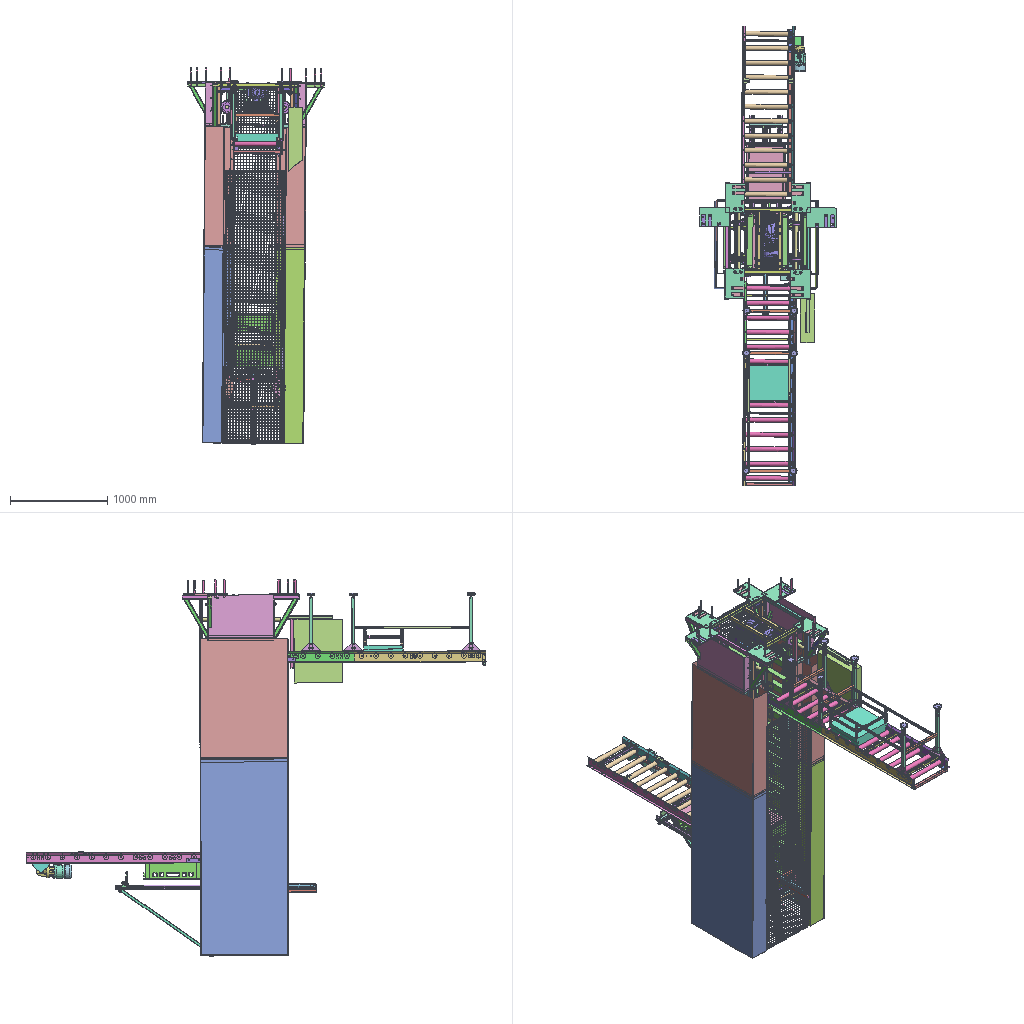Assembly | STEP file | 200 different items | 4291 placed | box 1401 x 4723 x 3865 mm
Parts list (item | name | quantity | parent item | size | volume):
1 | C3 | x2 | in Assembly1 | 298.717 x 900 x 1230 mm | 3124708 mm3
2 | C1 | x1 | in Assembly1 | 298.717 x 900 x 2010 mm | 4692484 mm3
3 | C1L | x1 | in Assembly1 | 298.717 x 900 x 2010 mm | 4679117 mm3
4 | C4 | x2 | in Assembly1 | 680 x 80 x 440 mm | 536518 mm3
5 | C4 connector | x2 | in Assembly1 | 677 x 48.5 x 50 mm | 57745 mm3
6 | Connector | x2 | in Assembly1 | 197.5 x 897 x 50 mm | 111605 mm3
7 | DIN EN 10210-2 - 20 x 20 x 2 - 2500 | x2 | in OS_00_01 | 20 x 20 x 2800 mm | 388388 mm3
8 | DIN EN 10210-2 - 20 x 20 x 2 - 1000 | x6 | in OS_00_01, OS_00_05, OS_00_06 | 20 x 20 x 610 mm | 82428 mm3
9 | JIS G 3191A - 6-1 | x199 | in OS_00_01, OS_00_05, OS_00_06 | 4 x 4 x 610 mm | 7665 mm3
10 | JIS G 3191A - 6-2 | x20 | in OS_00_01 | 4 x 4 x 2800 mm | 35186 mm3
11 | 1 | x2 | in OS_00_05 | 20 x 20 x 1000 mm | 136914 mm3
12 | P1 | x20 | in OS_00_05 | 4 x 4 x 1000 mm | 12566 mm3
13 | 2 | x2 | in OS_00_06 | 20 x 20 x 2200 mm | 304563 mm3
14 | P2 | x20 | in OS_00_06 | 4 x 4 x 2200 mm | 27646 mm3
15 | Channel 50x30x2x3-250 GOST 8278-83 | x1 | in Assembly2 | 40 x 45 x 250 mm | 58023 mm3
16 | DIN 59 410 - 40x40x2.9-500 | x1 | in Assembly2 | 40 x 40 x 470 mm | 187371 mm3
17 | DIN 59 410 - 40x40x2.9-300 | x1 | in Assembly2 | 40 x 40 x 500 mm | 194610 mm3
18 | Side panel wer5 N1 | x1 | in TR-1-Filet | 107.981 x 30 x 1800 mm | 501460 mm3
19 | Connector crossbar | x6 | in Crossbar | 48 x 3 x 60 mm | 7233 mm3
20 | DIN EN 10305-5 - 35 x 20 x 2  - 454 | x3 | in Crossbar | 20 x 30 x 475 mm | 84138 mm3
21 | Support gearmotor part2 B | x1 | in Gearmotor left | 94 x 194.451 x 110.566 mm | 79699 mm3
22 | Support gearmotor part1 B | x1 | in Gearmotor left | 180 x 89 x 30 mm | 35388 mm3
23 | Shaft1 | x1 | in 156 | 149.35 x 24 x 24 mm | 50304 mm3
24 | Roller 9 ribbed 2 | x1 | in Gearmotor left | 43.308 x 25.164 x 43.308 mm | 25808 mm3
25 | ISO 2491 - A  6 x 4 x 32 | x2 | in Keyed joint1 | 32 x 6 x 4 mm | 725.895 mm3
26 | 1 | x1 | in 3D_SK1SMI40AZ-IEC71-71L4_0,37KW | 135.85 x 125.7 x 192.425 mm | 2018687 mm3
27 | 2 | x1 | in 3D_SK1SMI40AZ-IEC71-71L4_0,37KW | 3.5 x 8 x 8 mm | 175.929 mm3
28 | 3 | x1 | in 3D_SK1SMI40AZ-IEC71-71L4_0,37KW | 3.5 x 8 x 8 mm | 175.929 mm3
29 | 4 | x1 | in 3D_SK1SMI40AZ-IEC71-71L4_0,37KW | 8 x 8 x 3.5 mm | 175.929 mm3
30 | 5 | x1 | in 3D_SK1SMI40AZ-IEC71-71L4_0,37KW | 8 x 8 x 3.5 mm | 175.929 mm3
31 | 6 | x1 | in 3D_SK1SMI40AZ-IEC71-71L4_0,37KW | 137.76 x 71.5 x 137.76 mm | 961193 mm3
32 | 7 | x1 | in 3D_SK1SMI40AZ-IEC71-71L4_0,37KW | 131 x 185.7 x 155.5 mm | 1497643 mm3
33 | DIN 9021 - 8,4 | x1 | in Gearmotor left | 2 x 24 x 24 mm | 793.943 mm3
34 | DIN 933 - M8  x 8 | x1 | in Gearmotor left | 13.3 x 15.011 x 13 mm | 1114 mm3
35 | Guard belt | x1 | in TR-1-Filet | 75 x 33.917 x 1461 mm | 248061 mm3
36 | Guard wheel drive wer2 | x1 | in TR-1-Filet | 245 x 88.5 x 68.5 mm | 32228 mm3
37 | Bracket for support | x2 | in TR-1-Filet | 45.331 x 61.284 x 200 mm | 31041 mm3
38 | Side panel wer5 N1 mirror | x1 | in TR-1-Filet | 107.981 x 30 x 1800 mm | 501354 mm3
39 | Guard wheel drive wer2 part2 | x1 | in TR-1-Filet | 245 x 120.904 x 13.322 mm | 29188 mm3
40 | Drive roller PolyV 420 mm | x12 | in TR-1-Filet | 49.999 x 500 x 49.999 mm | 924230 mm3
41 | Connector TR lift wer2 | x4 | in TR-1-Filet, QZ | 200 x 145 x 48 mm | 75134 mm3
42 | Side panel wer5 BeforeLift N7 | x1 | in Roller powered BeforeLift | 107.981 x 30 x 750 mm | 209231 mm3
43 | Side panel wer5 BeforeLift N7 mirror | x1 | in Roller powered BeforeLift | 107.981 x 30 x 750 mm | 208984 mm3
44 | Connector crossbar | x8 | in Crossbar | 48 x 3 x 60 mm | 7233 mm3
45 | DIN EN 10305-5 - 35 x 20 x 2  - 454 | x4 | in Crossbar | 20 x 30 x 475 mm | 83922 mm3
46 | Mounting leg part1 | x6 | in Roller powered BeforeLift, Roller gravity BeforeLift | 104.175 x 22.016 x 200 mm | 43311 mm3
47 | Leg 30x30x2 | x6 | in Roller powered BeforeLift, Roller gravity BeforeLift | 30 x 30 x 538 mm | 122015 mm3
48 | Leg crossbar 30x30x2 | x3 | in Roller powered BeforeLift, Roller gravity BeforeLift | 30 x 30 x 456 mm | 99013 mm3
49 | Levelling elements for ground mounting LV.F-80-14-SST-M12x98(0) | x6 | in Roller powered BeforeLift, Roller gravity BeforeLift | 80 x 131 x 80 mm | 93334 mm3
50 | Drive roller PolyV 420 mm | x14 | in Roller powered BeforeLift, Roller gravity BeforeLift | 49.999 x 500 x 49.999 mm | 924230 mm3
51 | Z-081D | x1 | in Roller powered BeforeLift | 46 x 60 x 2.9 mm | 7421 mm3
52 | Side panel wer5 BeforeLift gravity | x1 | in Roller gravity BeforeLift | 107.981 x 30 x 1350 mm | 376755 mm3
53 | Side panel wer5 BeforeLift gravity mirror | x1 | in Roller gravity BeforeLift | 107.981 x 30 x 1350 mm | 376614 mm3
54 | Mounting bumper | x2 | in Roller gravity BeforeLift | 120 x 30 x 4 mm | 13947 mm3
55 | DIN EN 10305-5 - 30 x 30 x 2  - 473 | x1 | in Roller gravity BeforeLift | 30 x 30 x 473 mm | 102704 mm3
56 | Guard belt Before lift | x1 | in Roller gravity BeforeLift | 75 x 33.917 x 2005 mm | 340463 mm3
57 | DIN EN 10210-2 - 20 x 20 x 2 - 500 | x2 | in QZ | 20 x 20 x 1180 mm | 164855 mm3
58 | DIN EN 10210-2 - 20 x 20 x 2 - 400 | x4 | in QZ | 20 x 20 x 400 mm | 55883 mm3
59 | Part3 | x1 | in QZ | 440 x 400 x 100 mm | 16640000 mm3
60 | DIN EN 10210-2 - 20 x 20 x 2 - 100 | x8 | in QZ | 20 x 20 x 75 mm | 10478 mm3
61 | Sheet29 | x8 | in IN_PRC_00_04, IN_PRC_00_03 | 160 x 156 x 56.288 mm | 49225 mm3
62 | DIN 126 - 9 | x143 | in IN_PRC_00_04, IN_PRC_00_03, P_01, Conveyor1, IN_AB_00_01, Conveyor | 16 x 16 x 1.6 mm | 219.911 mm3
63 | DIN 933 - M8  x 20 | x20 | in IN_PRC_00_04, IN_PRC_00_03, Conveyor1 | 25.3 x 15.011 x 13 mm | 1718 mm3
64 | DIN 128 - A8 | x77 | in IN_PRC_00_04, IN_PRC_00_03, P_01, Conveyor1, IN_AB_00_01, Conveyor | 1.6 x 14.8 x 14.8 mm | 178.348 mm3
65 | DIN 934 - M8 x 1,25 | x74 | in IN_PRC_00_04, IN_PRC_00_03, P_01, IN_AB_00_01, Conveyor | 6.5 x 15.011 x 13 mm | 685.442 mm3
66 | DIN 59 410 - 40x40x2.9-200 | x4 | in IN_PW_00_02, IN_PW_00_01 | 40 x 40 x 160 mm | 65392 mm3
67 | Shaft1 | x2 | in 156 | 272 x 25 x 25 mm | 113038 mm3
68 | Sheet34 | x8 | in IN_PW_00_02, IN_PW_00_01 | 34 x 34 x 10 mm | 6171 mm3
69 | 29020-30 | x8 | in IN_PW_00_02, IN_PW_00_01 | 72 x 47 x 22 mm | 32171 mm3
70 | Shaft2 | x2 | in 70 | 240 x 25 x 25 mm | 103493 mm3
71 | Plate | x4 | in P_01 | 88 x 350 x 10 mm | 290184 mm3
72 | DIN 7991 - M8  x  60 | x8 | in P_01 | 60 x 15.24 x 15.24 mm | 3321 mm3
73 | DIN 931-1 - M8 x 60 | x8 | in P_01 | 65.3 x 15.011 x 13 mm | 3758 mm3
74 | S3 | x4 | in P_01 | 114 x 200 x 33.288 mm | 36556 mm3
75 | Housing | x8 | in P_01 | 28 x 70 x 65 mm | 87955 mm3
76 | S3_MIR | x4 | in P_01 | 114 x 200 x 33.288 mm | 36556 mm3
77 | DIN 59 410 - 40x40x2.9-400 | x4 | in Conveyor frame | 40 x 40 x 350 mm | 142308 mm3
78 | DIN 59 410 - PPTM_02 | x4 | in Conveyor frame | 40 x 40 x 140 mm | 55897 mm3
79 | Sheet18 | x29 | in Conveyor frame, IN_ZA_00_01, IN_ZB_00_01, IN_ZC_00_01, IN_ZD_00_01, Assembly10, R1_01_rama | 34 x 34 x 3 mm | 3157 mm3
80 | 900 Mold To Width Flush Grid | x98 | in T_01 | 36.002 x 191.5 x 16.69 mm | 24114 mm3
81 | s3d9xxcjk1ng | x12 | in T_01 | 108.897 x 108.897 x 38.1 mm | 73401 mm3
82 | SK1SMI40AZH-IEC63-63L(1) | x2 | in Conveyor1, Conveyor | 181.38 x 343.8 x 154.88 mm | 3328871 mm3
83 | - | x1 | in Conveyor1 | 48 x 45 x 45 mm | 50486 mm3
84 | Roller chain1 | x1 | in Chain drive1 | 199.55 x 211.673 x 19.6 mm | 116843 mm3
85 | Roller chain sprocket11 | x1 | in Chain drive1 | 87.888 x 87.888 x 9.168 mm | 42964 mm3
86 | Roller chain sprocket21 | x1 | in Chain drive1 | 87.888 x 87.888 x 9.168 mm | 42964 mm3
87 | S | x1 | in Stasin guard return01 | 142.095 x 652.75 x 500 mm | 42330846 mm3
88 | DIN 59 410 - 40x40x2.9-800_L | x1 | in IN_ZA_00_01 | 40 x 40 x 590 mm | 239994 mm3
89 | Sheet10 | x1 | in IN_ZA_00_01 | 240 x 250 x 10 mm | 535218 mm3
90 | DIN 59 410 - 40x40x2.9-600 | x2 | in IN_ZA_00_01 | 40 x 40 x 795 mm | 317936 mm3
91 | DIN 59 410 - 60x60x2.9-600_1_L | x1 | in IN_ZA_00_01 | 40 x 40 x 715 mm | 290473 mm3
92 | Sheet1 | x4 | in IN_ZA_00_01 | 180 x 110 x 5 mm | 95551 mm3
93 | DIN 59 410 - 40x40x2.9-800 | x1 | in IN_ZA_00_01 | 40 x 40 x 590 mm | 240323 mm3
94 | DIN2448 - 17,2 x 2 - 40 | x68 | in IN_ZA_00_01, IN_ZB_00_01, IN_ZC_00_01, IN_ZD_00_01 | 17.2 x 17.2 x 40 mm | 3820 mm3
95 | Sheet19 | x10 | in IN_ZA_00_01, IN_ZC_00_01, IN_ZD_00_01 | 34 x 34 x 3 mm | 2909 mm3
96 | DIN 126 - 13,5 | x216 | in IN_ZA_00_01, IN_AB_00_01, IN_ZB_00_01, IN_ZC_00_01, IN_ZD_00_01 | 24 x 24 x 2.5 mm | 773.126 mm3
97 | DIN 128 - A12 | x128 | in IN_ZA_00_01, IN_AB_00_01, IN_ZB_00_01, IN_ZC_00_01, IN_ZD_00_01 | 2.1 x 21.1 x 21.1 mm | 443.477 mm3
98 | DIN 931-1 - M12 x 100 | x48 | in IN_ZA_00_01, IN_ZC_00_01, IN_ZD_00_01 | 107.5 x 21.939 x 19 mm | 13582 mm3
99 | DIN 934 - M12 x 1,75 | x128 | in IN_ZA_00_01, IN_AB_00_01, IN_ZB_00_01, IN_ZC_00_01, IN_ZD_00_01 | 10 x 21.939 x 19 mm | 2235 mm3
100 | DIN 126 - 15,5 | x8 | in IN_ZA_00_01 | 28 x 28 x 2.5 mm | 1068 mm3
101 | DIN 931-1 - M14 x 90 | x2 | in IN_ZA_00_01 | 98.8 x 25.403 x 22 mm | 17447 mm3
102 | DIN 931-1 - M14 x 50 | x2 | in IN_ZA_00_01 | 58.8 x 25.403 x 22 mm | 11289 mm3
103 | DIN 128 - A14 | x4 | in IN_ZA_00_01 | 2.4 x 24.1 x 24.1 mm | 656.6 mm3
104 | DIN 934 - M14 x 2 | x4 | in IN_ZA_00_01 | 11 x 25.403 x 22 mm | 3279 mm3
105 | DIN 59 410 - 60x60x2.9-600_1 | x10 | in IN_AB_00_01 | 40 x 40 x 584 mm | 236623 mm3
106 | Sheet6 | x20 | in IN_AB_00_01 | 180 x 50 x 8 mm | 68457 mm3
107 | DIN 931-1 - M8 x 65 | x40 | in IN_AB_00_01 | 70.3 x 15.011 x 13 mm | 4009 mm3
108 | DIN 9021 - 13 | x40 | in IN_AB_00_01 | 3 x 37 x 37 mm | 2827 mm3
109 | DIN 933 - M12  x 70 | x40 | in IN_AB_00_01 | 77.5 x 21.939 x 19 mm | 10105 mm3
110 | DIN 59 410 - 40x40x2.9-180_2 | x20 | in IN_ZB_00_01 | 40 x 40 x 100 mm | 40287 mm3
111 | DIN 59 410 - 40x40x2.9-2500 | x4 | in IN_ZB_00_01 | 40 x 40 x 3250 mm | 1317285 mm3
112 | DIN 59 410 - 40x40x2.9-180 | x4 | in IN_ZB_00_01 | 40 x 40 x 100 mm | 37023 mm3
113 | DIN 59 410 - 40x40x2.9-180_1 | x4 | in IN_ZB_00_01 | 40 x 40 x 100 mm | 38931 mm3
114 | DIN 59 410 - 40x40x2.9-2500_1 | x4 | in IN_ZB_00_01 | 40 x 40 x 3250 mm | 1322181 mm3
115 | DIN 931-1 - M12 x 70 | x32 | in IN_ZB_00_01 | 77.5 x 21.939 x 19 mm | 10189 mm3
116 | Shaft11 | x2 | in IN_S1_00_01 | 816.1 x 35 x 35 mm | 780993 mm3
117 | single_steel_sprocket_step_19_05mm_pgs19022m | x8 | in IN_S1_00_01, IN_S2_00_01, IN_S6_00_01 | 40 x 141.8 x 140.357 mm | 249105 mm3
118 | Shaft1 | x1 | in Shaft4 | 865 x 35 x 35 mm | 826461 mm3
119 | single_steel_sprocket_step_31_75mm_pgs31720m | x1 | in IN_S2_00_01 | 50 x 218.1 x 218.1 mm | 860633 mm3
120 | Shaft3 | x1 | in IN_S6_00_01 | 865 x 35 x 35 mm | 828041 mm3
121 | - | x1 | in 20_20B-35_1 | 83 x 75 x 75 mm | 165689 mm3
122 | single_steel_sprocket_step_31_75mm_pgs31720mBK | x1 | in 20_20B-35_1 | 51 x 218.1 x 218.1 mm | 824761 mm3
123 | Roller RB-19-12 10 | x112 | in IN_R1_00_01 | 28 x 28 x 23 mm | 11236 mm3
124 | Channel 25x26x2x3-50 GOST 8278-83 | x56 | in IN_R1_00_01 | 34 x 25 x 101 mm | 9812 mm3
125 | ANSI B18.3.3M - M8x1,25 x 29,25(2) | x112 | in IN_R1_00_01 | 36.25 x 16 x 16 mm | 3128 mm3
126 | DIN 125-2 - B 8,4A | x112 | in IN_R1_00_01 | 1.6 x 16 x 16 mm | 233.031 mm3
127 | DIN 934 - M8 x 1,25 | x114 | in IN_R1_00_01, GRC_01 | 6.5 x 15.011 x 13 mm | 685.442 mm3
128 | Angle bracket 1 | x28 | in IN_CZ_00_01 | 74.017 x 548.705 x 83.447 mm | 217025 mm3
129 | DIN 7991 - M6x16 | x224 | in IN_CZ_00_01, IN_C2_00_01 | 12 x 12 x 16 mm | 554.104 mm3
130 | DIN 126 - 6,6 | x296 | in IN_CZ_00_01, IN_C2_00_01, IN_PL_00_01, IN_PL_00_01_1 | 12 x 12 x 1.6 mm | 126.217 mm3
131 | DIN 934 - M6 x 1 | x296 | in IN_CZ_00_01, IN_C2_00_01, IN_PL_00_01, IN_PL_00_01_1 | 5 x 11.547 x 10 mm | 321.24 mm3
132 | 12b-1_01 | x112 | in 12b-1 | 33.5 x 14.5 x 22.6 mm | 2362 mm3
133 | 12b-1_02 | x112 | in 12b-1 | 35 x 15.9 x 15.6 mm | 2080 mm3
134 | 12b-1_03 | x112 | in 12b-1 | 12.07 x 12.07 x 11.6 mm | 683.04 mm3
135 | 12b-1_04 | x112 | in 12b-1 | 12.07 x 12.07 x 11.6 mm | 683.04 mm3
136 | 12b-1_05 | x112 | in 12b-1 | 35 x 15.9 x 15.6 mm | 2080 mm3
137 | 12b-1_06 | x112 | in 12b-1 | 12.07 x 12.07 x 11.6 mm | 683.04 mm3
138 | 12b-1_07 | x112 | in 12b-1 | 12.07 x 12.07 x 11.6 mm | 683.04 mm3
139 | 12b-1_e-1k2 | x56 | in 12B-Chain | 19.15 x 35.35 x 39.1 mm | 3982 mm3
140 | Sheet20 | x2 | in IN_ZC_00_01 | 300 x 200 x 12 mm | 698741 mm3
141 | DIN 59 410 - 40x40x2.9-400 | x8 | in IN_ZC_00_01, IN_ZD_00_01 | 40 x 40 x 495.189 mm | 183493 mm3
142 | Sheet5 | x6 | in IN_ZC_00_01, IN_ZD_00_01 | 300 x 200 x 12 mm | 645514 mm3
143 | DIN 59 410 - 40x40x2.9-300 | x8 | in IN_ZC_00_01, IN_ZD_00_01 | 40 x 40 x 550 mm | 219599 mm3
144 | DIN 59 410 - 40x40x2.9-800_DR | x3 | in IN_ZC_00_01, IN_ZD_00_01 | 40 x 40 x 795 mm | 317808 mm3
145 | DIN 933 - M12  x 40 | x8 | in IN_ZC_00_01, IN_ZD_00_01 | 47.5 x 21.939 x 19 mm | 6712 mm3
146 | Sheet21 | x16 | in IN_ZC_00_01, IN_ZD_00_01 | 300 x 200 x 3 mm | 150236 mm3
147 | DIN 59 410 - 40x40x2.9-1000_1 | x1 | in IN_ZC_00_01 | 40 x 40 x 900 mm | 366857 mm3
148 | DIN 59 410 - 40x40x2.9-1000_L | x1 | in IN_ZC_00_01 | 40 x 40 x 900 mm | 366857 mm3
149 | DIN 59 410 - 40x40x2.9-800_DR_01 | x1 | in IN_ZC_00_01 | 40 x 40 x 1400 mm | 564745 mm3
150 | tige_m12_nf_e_27_801_ecrou_h_01 | x24 | in tige_m12_nf_e_27_801_ecrou_h | 12 x 12 x 180 mm | 20325 mm3
151 | tige_m12_nf_e_27_801_ecrou_h_02 | x24 | in tige_m12_nf_e_27_801_ecrou_h | 21.939 x 19 x 10 mm | 2279 mm3
152 | DIN 59 410 - 40x40x2.9-600_2 | x4 | in IN_ZC_00_01, IN_ZD_00_01 | 40 x 40 x 600 mm | 241926 mm3
153 | S1 | x2 | in Conveyor | 70 x 36 x 88.858 mm | 8824 mm3
154 | S2 | x2 | in Conveyor | 20 x 20 x 40 mm | 10297 mm3
155 | 10B-1 z16_1 | x2 | in Assembly4 | 30 x 88 x 88 mm | 91202 mm3
156 | Shaft1 | x1 | in 156 | 161 x 20 x 20 mm | 49512 mm3
157 | S5 | x1 | in Conveyor | 112 x 94 x 34.858 mm | 39851 mm3
158 | DIN 59 410 - 40x40x2.9-1000_ZD_01 | x1 | in IN_ZD_00_01 | 40 x 40 x 1200 mm | 489076 mm3
159 | DIN 59 410 - 40x40x2.9-1000_ZD_02 | x1 | in IN_ZD_00_01 | 40 x 40 x 1200 mm | 489076 mm3
160 | DIN 931-1 - M12 x 65 | x8 | in IN_ZD_00_01 | 72.5 x 21.939 x 19 mm | 9623 mm3
161 | 150290 FENG-32-KF---(GK) | x1 | in 150290 FENG-32-400-KF---(asm_0) | 97 x 50 x 125 mm | 293495 mm3
162 | 150290 FENG-32-400-KF---(JS) | x1 | in 150290 FENG-32-400-KF---(asm_0) | 90 x 45 x 1055 mm | 299074 mm3
163 | DIN-912 - M6x30(F) | x4 | in 150290 FENG-32-400-KF---(asm_0) | 10 x 36 x 10 mm | 1236 mm3
164 | 160884 CRDNG-32-900-PPV-A---(ZR) | x1 | in 160884 CRDNG-32-700-PPV-A---(0) | 53 x 50 x 1014 mm | 321289 mm3
165 | 160884 CRDNG-32-400-PPV-A---(KS) | x2 | in 160884 CRDNG-32-700-PPV-A---(0), 160884 CRDNG-32-400-PPV-A---(0) | 32 x 32 x 991.817 mm | 118704 mm3
166 | DIN-439-B - M10x1_25(F) | x2 | in 160884 CRDNG-32-700-PPV-A---(0), 160884 CRDNG-32-400-PPV-A---(0) | 17 x 5 x 19.63 mm | 939.092 mm3
167 | JIS G 3350A - 1053     40x40x40-100 | x1 | in Lift no.3 | 55 x 105 x 125 mm | 75030 mm3
168 | DIN EN 10210-2 - 40 x 40 x 3 - 800 | x3 | in Assembly10 | 40 x 40 x 429 mm | 186333 mm3
169 | DIN EN 10210-2 - 20 x 20 x 2 - 900 | x1 | in Assembly10 | 40 x 40 x 600 mm | 259682 mm3
170 | Part4 | x4 | in Assembly10 | 40 x 80 x 3 mm | 8756 mm3
171 | mocowanie | x20 | in IN_PL_00_01, IN_PL_00_01_1 | 74 x 70 x 160 mm | 69052 mm3
172 | Angle 85x35x4-2800 GOST 19772-93 | x4 | in IN_PL_00_01, IN_PL_00_01_1 | 32 x 105 x 2700 mm | 1063844 mm3
173 | DIN 128 - A6 | x36 | in IN_PL_00_01, IN_PL_00_01_1 | 1.3 x 11.8 x 11.8 mm | 96.442 mm3
174 | PE_01 | x4 | in IN_PL_00_01, IN_PL_00_01_1 | 31 x 10 x 2700 mm | 827532 mm3
175 | PE_03 | x4 | in IN_PL_00_01, IN_PL_00_01_1 | 25 x 20 x 2700 mm | 1341954 mm3
176 | SK5 | x4 | in IN_PL_00_01, IN_PL_00_01_1 | 38 x 31.5 x 2660 mm | 335418 mm3
177 | Channel 30x25x3x5-50 GOST 8278-83 | x20 | in Assembly6, Assembly6 1, Assembly6 2, Assembly6 3 | 70 x 53 x 75 mm | 24715 mm3
178 | Part6 | x4 | in Assembly6, Assembly6 1, Assembly6 2, Assembly6 3 | 75 x 2 x 2700 mm | 405000 mm3
179 | DIN EN 10210-2 - 20 x 20 x 2 - 300 | x1 | in Assembly7 | 30 x 30 x 330 mm | 71888 mm3
180 | CSN EN 10219-2 - 30 x 30 x 2  - 800 | x1 | in Assembly7 | 30 x 30 x 1108 mm | 232357 mm3
181 | Part1 | x4 | in Assembly7, R1_01_rama | 100 x 40 x 3 mm | 11365 mm3
182 | DIN 933 - M10  x 65 | x2 | in Lift no.3 | 71.4 x 19.63 x 17 mm | 6601 mm3
183 | Skrzynka_ver.1.1 | x2 | in Lift no.3 | 600 x 200 x 400 mm | 4256254 mm3
184 | DIN 933 - M6  x 60 | x4 | in Lift no.3 | 64 x 11.547 x 10 mm | 2012 mm3
185 | DIN 934 - M6 x 1 | x18 | in Lift no.3, GRC_01 | 5 x 11.547 x 10 mm | 321.24 mm3
186 | b7-ashw-16-1000 | x2 | in GRC_01 | 48 x 38 x 1000 mm | 648601 mm3
187 | b92-gnkso-16-ppas | x2 | in GRC_01 | 37 x 35 x 53 mm | 52576 mm3
188 | wer4r34e | x1 | in GRC_01 | 65 x 15 x 90 mm | 19731 mm3
189 | BS EN ISO 1127(2) - 12 x 1,6 - 100 | x1 | in GRC_01 | 12 x 12 x 90 mm | 4705 mm3
190 | Part5 | x1 | in GRC_01 | 291 x 121 x 16.288 mm | 71655 mm3
191 | DIN 933 - M6  x 40 | x4 | in GRC_01 | 44 x 11.547 x 10 mm | 1446 mm3
192 | CSN EN 10305-5 - 40 x 20 x 2  - 330 | x1 | in GRC_01 | 20 x 40 x 335 mm | 72739 mm3
193 | BS EN 10305-4 - E235 - 12 x 1,5 - 50 | x2 | in GRC_01 | 12 x 12 x 50 mm | 2474 mm3
194 | Rod1 | x1 | in GRC_01 | 8 x 8 x 210 mm | 10533 mm3
195 | PE06 | x1 | in GRC_01 | 411 x 105 x 10 mm | 292762 mm3
196 | DIN 7991 - M6  x  20 | x10 | in GRC_01 | 20 x 11.34 x 11.34 mm | 687.937 mm3
197 | R1_01_rama_Spoiny | x1 | in R1_01_rama | 50.98 x 559.497 x 372.642 mm | 5856 mm3
198 | 1 | x1 | in R1_01_rama | 40 x 40 x 397.182 mm | 149500 mm3
199 | 2 | x1 | in R1_01_rama | 40 x 40 x 370 mm | 154561 mm3
200 | 3 | x1 | in R1_01_rama | 40 x 40 x 520 mm | 217221 mm3
Placements (level | parent | child | x y z in mm | rotation matrix by rows), first 285 of 4684 lines:
1 | Stasin guard return01 | Assembly1 | -747.43 -374.311 61.133 | 1 0.005068 0.007537 -0.005087 1 0.002503 -0.007524 -0.002541 1
2 | Assembly1 | C3 | -830.914 -828.99 1135.117 | 1 0 0 0 -1 0 0 0 -1
2 | Assembly1 | C1 | -815.914 -828.99 150.117 | 1 0 0 0 -1 0 0 0 -1
2 | Assembly1 | C3 | 185.585 -828.99 405.117 | -1 0 0 0 -1 0 0 0 1
2 | Assembly1 | C1L | 170.585 -828.99 -1349.883 | -1 0 0 0 -1 0 0 0 1
2 | Assembly1 | C4 | 115.585 -56.49 1395.117 | 0 1 0 -1 0 0 0 0 1
2 | Assembly1 | C4 | -760.914 -736.49 1395.117 | 0 -1 0 1 0 0 0 0 1
2 | Assembly1 | C4 connector | -790.914 -736.49 1370.117 | 0 -1 0 1 0 0 0 0 1
2 | Assembly1 | C4 connector | 145.585 -736.49 1420.117 | 0 1 0 1 0 0 0 0 -1
2 | Assembly1 | Connector | -815.914 16.01 120.117 | 1 0 0 0 1 0 0 0 1
2 | Assembly1 | Connector | 170.585 16.01 180.117 | -1 0 0 0 1 0 0 0 -1
2 | Assembly1 | OS_00_01 | -545.958 -1034.13 -508.199 | 0 1 0 -1 0 0 0 0 1
3 | OS_00_01 | DIN EN 10210-2 - 20 x 20 x 2 - 2500 | -178.393 -68.956 -1351.684 | 1 0 0 0 1 0 0 0 1
3 | OS_00_01 | DIN EN 10210-2 - 20 x 20 x 2 - 2500 | -178.393 521.044 -1351.684 | -1 0 0 0 -1 0 0 0 1
3 | OS_00_01 | DIN EN 10210-2 - 20 x 20 x 2 - 1000 | -178.393 -78.956 -1341.684 | -1 0 0 0 0 1 0 1 -0
3 | OS_00_01 | DIN EN 10210-2 - 20 x 20 x 2 - 1000 | -178.393 -78.956 1438.316 | 1 0 0 0 0 1 0 -1 0
3 | OS_00_01 | JIS G 3191A - 6-1 | -166.393 531.044 -1321.684 | 1 0 0 0 0 -1 0 1 0
3 | OS_00_01 | JIS G 3191A - 6-1 | -166.393 531.044 -1291.684 | 1 0 0 0 0 -1 0 1 0
3 | OS_00_01 | JIS G 3191A - 6-1 | -166.393 531.044 -1261.684 | 1 0 0 0 0 -1 0 1 0
3 | OS_00_01 | JIS G 3191A - 6-1 | -166.393 531.044 -1231.684 | 1 0 0 0 0 -1 0 1 0
3 | OS_00_01 | JIS G 3191A - 6-1 | -166.393 531.044 -1201.684 | 1 0 0 0 0 -1 0 1 0
3 | OS_00_01 | JIS G 3191A - 6-1 | -166.393 531.044 -1171.684 | 1 0 0 0 0 -1 0 1 0
3 | OS_00_01 | JIS G 3191A - 6-1 | -166.393 531.044 -1141.684 | 1 0 0 0 0 -1 0 1 0
3 | OS_00_01 | JIS G 3191A - 6-1 | -166.393 531.044 -1111.684 | 1 0 0 0 0 -1 0 1 0
3 | OS_00_01 | JIS G 3191A - 6-1 | -166.393 531.044 -1081.684 | 1 0 0 0 0 -1 0 1 0
3 | OS_00_01 | JIS G 3191A - 6-1 | -166.393 531.044 -1051.684 | 1 0 0 0 0 -1 0 1 0
3 | OS_00_01 | JIS G 3191A - 6-1 | -166.393 531.044 -1021.684 | 1 0 0 0 0 -1 0 1 0
3 | OS_00_01 | JIS G 3191A - 6-1 | -166.393 531.044 -991.684 | 1 0 0 0 0 -1 0 1 0
3 | OS_00_01 | JIS G 3191A - 6-1 | -166.393 531.044 -961.684 | 1 0 0 0 0 -1 0 1 0
3 | OS_00_01 | JIS G 3191A - 6-1 | -166.393 531.044 -931.684 | 1 0 0 0 0 -1 0 1 0
3 | OS_00_01 | JIS G 3191A - 6-1 | -166.393 531.044 -901.684 | 1 0 0 0 0 -1 0 1 0
3 | OS_00_01 | JIS G 3191A - 6-1 | -166.393 531.044 -871.684 | 1 0 0 0 0 -1 0 1 0
3 | OS_00_01 | JIS G 3191A - 6-1 | -166.393 531.044 -841.684 | 1 0 0 0 0 -1 0 1 0
3 | OS_00_01 | JIS G 3191A - 6-1 | -166.393 531.044 -811.684 | 1 0 0 0 0 -1 0 1 0
3 | OS_00_01 | JIS G 3191A - 6-1 | -166.393 531.044 -781.684 | 1 0 0 0 0 -1 0 1 0
3 | OS_00_01 | JIS G 3191A - 6-1 | -166.393 531.044 -751.684 | 1 0 0 0 0 -1 0 1 0
3 | OS_00_01 | JIS G 3191A - 6-1 | -166.393 531.044 -721.684 | 1 0 0 0 0 -1 0 1 0
3 | OS_00_01 | JIS G 3191A - 6-1 | -166.393 531.044 -691.684 | 1 0 0 0 0 -1 0 1 0
3 | OS_00_01 | JIS G 3191A - 6-1 | -166.393 531.044 -661.684 | 1 0 0 0 0 -1 0 1 0
3 | OS_00_01 | JIS G 3191A - 6-1 | -166.393 531.044 -631.684 | 1 0 0 0 0 -1 0 1 0
3 | OS_00_01 | JIS G 3191A - 6-1 | -166.393 531.044 -601.684 | 1 0 0 0 0 -1 0 1 0
3 | OS_00_01 | JIS G 3191A - 6-1 | -166.393 531.044 -571.684 | 1 0 0 0 0 -1 0 1 0
3 | OS_00_01 | JIS G 3191A - 6-1 | -166.393 531.044 -541.684 | 1 0 0 0 0 -1 0 1 0
3 | OS_00_01 | JIS G 3191A - 6-1 | -166.393 531.044 -511.684 | 1 0 0 0 0 -1 0 1 0
3 | OS_00_01 | JIS G 3191A - 6-1 | -166.393 531.044 -481.684 | 1 0 0 0 0 -1 0 1 0
3 | OS_00_01 | JIS G 3191A - 6-1 | -166.393 531.044 -451.684 | 1 0 0 0 0 -1 0 1 0
3 | OS_00_01 | JIS G 3191A - 6-1 | -166.393 531.044 -421.684 | 1 0 0 0 0 -1 0 1 0
3 | OS_00_01 | JIS G 3191A - 6-1 | -166.393 531.044 -391.684 | 1 0 0 0 0 -1 0 1 0
3 | OS_00_01 | JIS G 3191A - 6-1 | -166.393 531.044 -361.684 | 1 0 0 0 0 -1 0 1 0
3 | OS_00_01 | JIS G 3191A - 6-1 | -166.393 531.044 -331.684 | 1 0 0 0 0 -1 0 1 0
3 | OS_00_01 | JIS G 3191A - 6-1 | -166.393 531.044 -301.684 | 1 0 0 0 0 -1 0 1 0
3 | OS_00_01 | JIS G 3191A - 6-1 | -166.393 531.044 -271.684 | 1 0 0 0 0 -1 0 1 0
3 | OS_00_01 | JIS G 3191A - 6-1 | -166.393 531.044 -241.684 | 1 0 0 0 0 -1 0 1 0
3 | OS_00_01 | JIS G 3191A - 6-1 | -166.393 531.044 -211.684 | 1 0 0 0 0 -1 0 1 0
3 | OS_00_01 | JIS G 3191A - 6-1 | -166.393 531.044 -181.684 | 1 0 0 0 0 -1 0 1 0
3 | OS_00_01 | JIS G 3191A - 6-1 | -166.393 531.044 -151.684 | 1 0 0 0 0 -1 0 1 0
3 | OS_00_01 | JIS G 3191A - 6-1 | -166.393 531.044 -121.684 | 1 0 0 0 0 -1 0 1 0
3 | OS_00_01 | JIS G 3191A - 6-1 | -166.393 531.044 -91.684 | 1 0 0 0 0 -1 0 1 0
3 | OS_00_01 | JIS G 3191A - 6-1 | -166.393 531.044 -61.684 | 1 0 0 0 0 -1 0 1 0
3 | OS_00_01 | JIS G 3191A - 6-1 | -166.393 531.044 -31.684 | 1 0 0 0 0 -1 0 1 0
3 | OS_00_01 | JIS G 3191A - 6-1 | -166.393 531.044 -1.684 | 1 0 0 0 0 -1 0 1 0
3 | OS_00_01 | JIS G 3191A - 6-1 | -166.393 531.044 28.316 | 1 0 0 0 0 -1 0 1 0
3 | OS_00_01 | JIS G 3191A - 6-1 | -166.393 531.044 58.316 | 1 0 0 0 0 -1 0 1 0
3 | OS_00_01 | JIS G 3191A - 6-1 | -166.393 531.044 88.316 | 1 0 0 0 0 -1 0 1 0
3 | OS_00_01 | JIS G 3191A - 6-1 | -166.393 531.044 118.316 | 1 0 0 0 0 -1 0 1 0
3 | OS_00_01 | JIS G 3191A - 6-1 | -166.393 531.044 148.316 | 1 0 0 0 0 -1 0 1 0
3 | OS_00_01 | JIS G 3191A - 6-1 | -166.393 531.044 178.316 | 1 0 0 0 0 -1 0 1 0
3 | OS_00_01 | JIS G 3191A - 6-1 | -166.393 531.044 208.316 | 1 0 0 0 0 -1 0 1 0
3 | OS_00_01 | JIS G 3191A - 6-1 | -166.393 531.044 238.316 | 1 0 0 0 0 -1 0 1 0
3 | OS_00_01 | JIS G 3191A - 6-1 | -166.393 531.044 268.316 | 1 0 0 0 0 -1 0 1 0
3 | OS_00_01 | JIS G 3191A - 6-1 | -166.393 531.044 298.316 | 1 0 0 0 0 -1 0 1 0
3 | OS_00_01 | JIS G 3191A - 6-1 | -166.393 531.044 328.316 | 1 0 0 0 0 -1 0 1 0
3 | OS_00_01 | JIS G 3191A - 6-1 | -166.393 531.044 358.316 | 1 0 0 0 0 -1 0 1 0
3 | OS_00_01 | JIS G 3191A - 6-1 | -166.393 531.044 388.316 | 1 0 0 0 0 -1 0 1 0
3 | OS_00_01 | JIS G 3191A - 6-1 | -166.393 531.044 418.316 | 1 0 0 0 0 -1 0 1 0
3 | OS_00_01 | JIS G 3191A - 6-1 | -166.393 531.044 448.316 | 1 0 0 0 0 -1 0 1 0
3 | OS_00_01 | JIS G 3191A - 6-1 | -166.393 531.044 478.316 | 1 0 0 0 0 -1 0 1 0
3 | OS_00_01 | JIS G 3191A - 6-1 | -166.393 531.044 508.316 | 1 0 0 0 0 -1 0 1 0
3 | OS_00_01 | JIS G 3191A - 6-1 | -166.393 531.044 538.316 | 1 0 0 0 0 -1 0 1 0
3 | OS_00_01 | JIS G 3191A - 6-1 | -166.393 531.044 568.316 | 1 0 0 0 0 -1 0 1 0
3 | OS_00_01 | JIS G 3191A - 6-1 | -166.393 531.044 598.316 | 1 0 0 0 0 -1 0 1 0
3 | OS_00_01 | JIS G 3191A - 6-1 | -166.393 531.044 628.316 | 1 0 0 0 0 -1 0 1 0
3 | OS_00_01 | JIS G 3191A - 6-1 | -166.393 531.044 658.316 | 1 0 0 0 0 -1 0 1 0
3 | OS_00_01 | JIS G 3191A - 6-1 | -166.393 531.044 688.316 | 1 0 0 0 0 -1 0 1 0
3 | OS_00_01 | JIS G 3191A - 6-1 | -166.393 531.044 718.316 | 1 0 0 0 0 -1 0 1 0
3 | OS_00_01 | JIS G 3191A - 6-1 | -166.393 531.044 748.316 | 1 0 0 0 0 -1 0 1 0
3 | OS_00_01 | JIS G 3191A - 6-1 | -166.393 531.044 778.316 | 1 0 0 0 0 -1 0 1 0
3 | OS_00_01 | JIS G 3191A - 6-1 | -166.393 531.044 808.316 | 1 0 0 0 0 -1 0 1 0
3 | OS_00_01 | JIS G 3191A - 6-1 | -166.393 531.044 838.316 | 1 0 0 0 0 -1 0 1 0
3 | OS_00_01 | JIS G 3191A - 6-1 | -166.393 531.044 868.316 | 1 0 0 0 0 -1 0 1 0
3 | OS_00_01 | JIS G 3191A - 6-1 | -166.393 531.044 898.316 | 1 0 0 0 0 -1 0 1 0
3 | OS_00_01 | JIS G 3191A - 6-1 | -166.393 531.044 928.316 | 1 0 0 0 0 -1 0 1 0
3 | OS_00_01 | JIS G 3191A - 6-1 | -166.393 531.044 958.316 | 1 0 0 0 0 -1 0 1 0
3 | OS_00_01 | JIS G 3191A - 6-1 | -166.393 531.044 988.316 | 1 0 0 0 0 -1 0 1 0
3 | OS_00_01 | JIS G 3191A - 6-1 | -166.393 531.044 1018.316 | 1 0 0 0 0 -1 0 1 0
3 | OS_00_01 | JIS G 3191A - 6-1 | -166.393 531.044 1048.316 | 1 0 0 0 0 -1 0 1 0
3 | OS_00_01 | JIS G 3191A - 6-1 | -166.393 531.044 1078.316 | 1 0 0 0 0 -1 0 1 0
3 | OS_00_01 | JIS G 3191A - 6-1 | -166.393 531.044 1108.316 | 1 0 0 0 0 -1 0 1 0
3 | OS_00_01 | JIS G 3191A - 6-1 | -166.393 531.044 1138.316 | 1 0 0 0 0 -1 0 1 0
3 | OS_00_01 | JIS G 3191A - 6-1 | -166.393 531.044 1168.316 | 1 0 0 0 0 -1 0 1 0
3 | OS_00_01 | JIS G 3191A - 6-1 | -166.393 531.044 1198.316 | 1 0 0 0 0 -1 0 1 0
3 | OS_00_01 | JIS G 3191A - 6-1 | -166.393 531.044 1228.316 | 1 0 0 0 0 -1 0 1 0
3 | OS_00_01 | JIS G 3191A - 6-1 | -166.393 531.044 1258.316 | 1 0 0 0 0 -1 0 1 0
3 | OS_00_01 | JIS G 3191A - 6-1 | -166.393 531.044 1288.316 | 1 0 0 0 0 -1 0 1 0
3 | OS_00_01 | JIS G 3191A - 6-1 | -166.393 531.044 1318.316 | 1 0 0 0 0 -1 0 1 0
3 | OS_00_01 | JIS G 3191A - 6-1 | -166.393 531.044 1348.316 | 1 0 0 0 0 -1 0 1 0
3 | OS_00_01 | JIS G 3191A - 6-1 | -166.393 531.044 1378.316 | 1 0 0 0 0 -1 0 1 0
3 | OS_00_01 | JIS G 3191A - 6-1 | -166.393 531.044 1408.316 | 1 0 0 0 0 -1 0 1 0
3 | OS_00_01 | JIS G 3191A - 6-1 | -166.393 531.044 1438.316 | 1 0 0 0 0 -1 0 1 0
3 | OS_00_01 | JIS G 3191A - 6-2 | -166.393 501.044 -1351.684 | 1 0 0 0 1 0 0 0 1
3 | OS_00_01 | JIS G 3191A - 6-2 | -166.393 471.044 -1351.684 | 1 0 0 0 1 0 0 0 1
3 | OS_00_01 | JIS G 3191A - 6-2 | -166.393 441.044 -1351.684 | 1 0 0 0 1 0 0 0 1
3 | OS_00_01 | JIS G 3191A - 6-2 | -166.393 411.044 -1351.684 | 1 0 0 0 1 0 0 0 1
3 | OS_00_01 | JIS G 3191A - 6-2 | -166.393 381.044 -1351.684 | 1 0 0 0 1 0 0 0 1
3 | OS_00_01 | JIS G 3191A - 6-2 | -166.393 351.044 -1351.684 | 1 0 0 0 1 0 0 0 1
3 | OS_00_01 | JIS G 3191A - 6-2 | -166.393 321.044 -1351.684 | 1 0 0 0 1 0 0 0 1
3 | OS_00_01 | JIS G 3191A - 6-2 | -166.393 291.044 -1351.684 | 1 0 0 0 1 0 0 0 1
3 | OS_00_01 | JIS G 3191A - 6-2 | -166.393 261.044 -1351.684 | 1 0 0 0 1 0 0 0 1
3 | OS_00_01 | JIS G 3191A - 6-2 | -166.393 231.044 -1351.684 | 1 0 0 0 1 0 0 0 1
3 | OS_00_01 | JIS G 3191A - 6-2 | -166.393 201.044 -1351.684 | 1 0 0 0 1 0 0 0 1
3 | OS_00_01 | JIS G 3191A - 6-2 | -166.393 171.044 -1351.684 | 1 0 0 0 1 0 0 0 1
3 | OS_00_01 | JIS G 3191A - 6-2 | -166.393 141.044 -1351.684 | 1 0 0 0 1 0 0 0 1
3 | OS_00_01 | JIS G 3191A - 6-2 | -166.393 111.044 -1351.684 | 1 0 0 0 1 0 0 0 1
3 | OS_00_01 | JIS G 3191A - 6-2 | -166.393 81.044 -1351.684 | 1 0 0 0 1 0 0 0 1
3 | OS_00_01 | JIS G 3191A - 6-2 | -166.393 51.044 -1351.684 | 1 0 0 0 1 0 0 0 1
3 | OS_00_01 | JIS G 3191A - 6-2 | -166.393 21.044 -1351.684 | 1 0 0 0 1 0 0 0 1
3 | OS_00_01 | JIS G 3191A - 6-2 | -166.393 -8.956 -1351.684 | 1 0 0 0 1 0 0 0 1
3 | OS_00_01 | JIS G 3191A - 6-2 | -166.393 -38.956 -1351.684 | 1 0 0 0 1 0 0 0 1
3 | OS_00_01 | JIS G 3191A - 6-2 | -166.393 -68.956 -1351.684 | 1 0 0 0 1 0 0 0 1
2 | Assembly1 | OS_00_05 | -93.871 191.903 -508.199 | 0 -1 0 1 0 0 0 0 1
3 | OS_00_05 | 1 | -178.393 -68.956 -1351.684 | 1 0 0 0 1 0 0 0 1
3 | OS_00_05 | 1 | -178.393 521.044 -1351.684 | -1 0 0 0 -1 0 0 0 1
3 | OS_00_05 | DIN EN 10210-2 - 20 x 20 x 2 - 1000 | -178.393 -78.956 -1341.684 | -1 0 0 0 0 1 0 1 -0
3 | OS_00_05 | DIN EN 10210-2 - 20 x 20 x 2 - 1000 | -178.393 -78.956 -361.684 | 1 0 0 0 0 1 0 -1 0
3 | OS_00_05 | JIS G 3191A - 6-1 | -166.393 531.044 -1321.684 | 1 0 0 0 0 -1 0 1 0
3 | OS_00_05 | JIS G 3191A - 6-1 | -166.393 531.044 -1291.684 | 1 0 0 0 0 -1 0 1 0
3 | OS_00_05 | JIS G 3191A - 6-1 | -166.393 531.044 -1261.684 | 1 0 0 0 0 -1 0 1 0
3 | OS_00_05 | JIS G 3191A - 6-1 | -166.393 531.044 -1231.684 | 1 0 0 0 0 -1 0 1 0
3 | OS_00_05 | JIS G 3191A - 6-1 | -166.393 531.044 -1201.684 | 1 0 0 0 0 -1 0 1 0
3 | OS_00_05 | JIS G 3191A - 6-1 | -166.393 531.044 -1171.684 | 1 0 0 0 0 -1 0 1 0
3 | OS_00_05 | JIS G 3191A - 6-1 | -166.393 531.044 -1141.684 | 1 0 0 0 0 -1 0 1 0
3 | OS_00_05 | JIS G 3191A - 6-1 | -166.393 531.044 -1111.684 | 1 0 0 0 0 -1 0 1 0
3 | OS_00_05 | JIS G 3191A - 6-1 | -166.393 531.044 -1081.684 | 1 0 0 0 0 -1 0 1 0
3 | OS_00_05 | JIS G 3191A - 6-1 | -166.393 531.044 -1051.684 | 1 0 0 0 0 -1 0 1 0
3 | OS_00_05 | JIS G 3191A - 6-1 | -166.393 531.044 -1021.684 | 1 0 0 0 0 -1 0 1 0
3 | OS_00_05 | JIS G 3191A - 6-1 | -166.393 531.044 -991.684 | 1 0 0 0 0 -1 0 1 0
3 | OS_00_05 | JIS G 3191A - 6-1 | -166.393 531.044 -961.684 | 1 0 0 0 0 -1 0 1 0
3 | OS_00_05 | JIS G 3191A - 6-1 | -166.393 531.044 -931.684 | 1 0 0 0 0 -1 0 1 0
3 | OS_00_05 | JIS G 3191A - 6-1 | -166.393 531.044 -901.684 | 1 0 0 0 0 -1 0 1 0
3 | OS_00_05 | JIS G 3191A - 6-1 | -166.393 531.044 -871.684 | 1 0 0 0 0 -1 0 1 0
3 | OS_00_05 | JIS G 3191A - 6-1 | -166.393 531.044 -841.684 | 1 0 0 0 0 -1 0 1 0
3 | OS_00_05 | JIS G 3191A - 6-1 | -166.393 531.044 -811.684 | 1 0 0 0 0 -1 0 1 0
3 | OS_00_05 | JIS G 3191A - 6-1 | -166.393 531.044 -781.684 | 1 0 0 0 0 -1 0 1 0
3 | OS_00_05 | JIS G 3191A - 6-1 | -166.393 531.044 -751.684 | 1 0 0 0 0 -1 0 1 0
3 | OS_00_05 | JIS G 3191A - 6-1 | -166.393 531.044 -721.684 | 1 0 0 0 0 -1 0 1 0
3 | OS_00_05 | JIS G 3191A - 6-1 | -166.393 531.044 -691.684 | 1 0 0 0 0 -1 0 1 0
3 | OS_00_05 | JIS G 3191A - 6-1 | -166.393 531.044 -661.684 | 1 0 0 0 0 -1 0 1 0
3 | OS_00_05 | JIS G 3191A - 6-1 | -166.393 531.044 -631.684 | 1 0 0 0 0 -1 0 1 0
3 | OS_00_05 | JIS G 3191A - 6-1 | -166.393 531.044 -601.684 | 1 0 0 0 0 -1 0 1 0
3 | OS_00_05 | JIS G 3191A - 6-1 | -166.393 531.044 -571.684 | 1 0 0 0 0 -1 0 1 0
3 | OS_00_05 | JIS G 3191A - 6-1 | -166.393 531.044 -541.684 | 1 0 0 0 0 -1 0 1 0
3 | OS_00_05 | JIS G 3191A - 6-1 | -166.393 531.044 -511.684 | 1 0 0 0 0 -1 0 1 0
3 | OS_00_05 | JIS G 3191A - 6-1 | -166.393 531.044 -481.684 | 1 0 0 0 0 -1 0 1 0
3 | OS_00_05 | JIS G 3191A - 6-1 | -166.393 531.044 -451.684 | 1 0 0 0 0 -1 0 1 0
3 | OS_00_05 | JIS G 3191A - 6-1 | -166.393 531.044 -421.684 | 1 0 0 0 0 -1 0 1 0
3 | OS_00_05 | JIS G 3191A - 6-1 | -166.393 531.044 -391.684 | 1 0 0 0 0 -1 0 1 0
3 | OS_00_05 | JIS G 3191A - 6-1 | -166.393 531.044 -361.684 | 1 0 0 0 0 -1 0 1 0
3 | OS_00_05 | P1 | -166.393 501.044 -1351.684 | 1 0 0 0 1 0 0 0 1
3 | OS_00_05 | P1 | -166.393 471.044 -1351.684 | 1 0 0 0 1 0 0 0 1
3 | OS_00_05 | P1 | -166.393 441.044 -1351.684 | 1 0 0 0 1 0 0 0 1
3 | OS_00_05 | P1 | -166.393 411.044 -1351.684 | 1 0 0 0 1 0 0 0 1
3 | OS_00_05 | P1 | -166.393 381.044 -1351.684 | 1 0 0 0 1 0 0 0 1
3 | OS_00_05 | P1 | -166.393 351.044 -1351.684 | 1 0 0 0 1 0 0 0 1
3 | OS_00_05 | P1 | -166.393 321.044 -1351.684 | 1 0 0 0 1 0 0 0 1
3 | OS_00_05 | P1 | -166.393 291.044 -1351.684 | 1 0 0 0 1 0 0 0 1
3 | OS_00_05 | P1 | -166.393 261.044 -1351.684 | 1 0 0 0 1 0 0 0 1
3 | OS_00_05 | P1 | -166.393 231.044 -1351.684 | 1 0 0 0 1 0 0 0 1
3 | OS_00_05 | P1 | -166.393 201.044 -1351.684 | 1 0 0 0 1 0 0 0 1
3 | OS_00_05 | P1 | -166.393 171.044 -1351.684 | 1 0 0 0 1 0 0 0 1
3 | OS_00_05 | P1 | -166.393 141.044 -1351.684 | 1 0 0 0 1 0 0 0 1
3 | OS_00_05 | P1 | -166.393 111.044 -1351.684 | 1 0 0 0 1 0 0 0 1
3 | OS_00_05 | P1 | -166.393 81.044 -1351.684 | 1 0 0 0 1 0 0 0 1
3 | OS_00_05 | P1 | -166.393 51.044 -1351.684 | 1 0 0 0 1 0 0 0 1
3 | OS_00_05 | P1 | -166.393 21.044 -1351.684 | 1 0 0 0 1 0 0 0 1
3 | OS_00_05 | P1 | -166.393 -8.956 -1351.684 | 1 0 0 0 1 0 0 0 1
3 | OS_00_05 | P1 | -166.393 -38.956 -1351.684 | 1 0 0 0 1 0 0 0 1
3 | OS_00_05 | P1 | -166.393 -68.956 -1351.684 | 1 0 0 0 1 0 0 0 1
2 | Assembly1 | OS_00_06 | -93.871 191.903 934.391 | 0 -1 0 1 0 0 0 0 1
3 | OS_00_06 | 2 | -178.393 -68.956 -1351.684 | 1 0 0 0 1 0 0 0 1
3 | OS_00_06 | 2 | -178.393 521.044 -1351.684 | -1 0 0 0 -1 0 0 0 1
3 | OS_00_06 | DIN EN 10210-2 - 20 x 20 x 2 - 1000 | -178.393 -78.956 -1341.684 | -1 0 0 0 0 1 0 1 -0
3 | OS_00_06 | DIN EN 10210-2 - 20 x 20 x 2 - 1000 | -178.393 -78.956 838.316 | 1 0 0 0 0 1 0 -1 0
3 | OS_00_06 | JIS G 3191A - 6-1 | -166.393 531.044 -1321.684 | 1 0 0 0 0 -1 0 1 0
3 | OS_00_06 | JIS G 3191A - 6-1 | -166.393 531.044 -1291.684 | 1 0 0 0 0 -1 0 1 0
3 | OS_00_06 | JIS G 3191A - 6-1 | -166.393 531.044 -1261.684 | 1 0 0 0 0 -1 0 1 0
3 | OS_00_06 | JIS G 3191A - 6-1 | -166.393 531.044 -1231.684 | 1 0 0 0 0 -1 0 1 0
3 | OS_00_06 | JIS G 3191A - 6-1 | -166.393 531.044 -1201.684 | 1 0 0 0 0 -1 0 1 0
3 | OS_00_06 | JIS G 3191A - 6-1 | -166.393 531.044 -1171.684 | 1 0 0 0 0 -1 0 1 0
3 | OS_00_06 | JIS G 3191A - 6-1 | -166.393 531.044 -1141.684 | 1 0 0 0 0 -1 0 1 0
3 | OS_00_06 | JIS G 3191A - 6-1 | -166.393 531.044 -1111.684 | 1 0 0 0 0 -1 0 1 0
3 | OS_00_06 | JIS G 3191A - 6-1 | -166.393 531.044 -1081.684 | 1 0 0 0 0 -1 0 1 0
3 | OS_00_06 | JIS G 3191A - 6-1 | -166.393 531.044 -1051.684 | 1 0 0 0 0 -1 0 1 0
3 | OS_00_06 | JIS G 3191A - 6-1 | -166.393 531.044 -1021.684 | 1 0 0 0 0 -1 0 1 0
3 | OS_00_06 | JIS G 3191A - 6-1 | -166.393 531.044 -991.684 | 1 0 0 0 0 -1 0 1 0
3 | OS_00_06 | JIS G 3191A - 6-1 | -166.393 531.044 -961.684 | 1 0 0 0 0 -1 0 1 0
3 | OS_00_06 | JIS G 3191A - 6-1 | -166.393 531.044 -931.684 | 1 0 0 0 0 -1 0 1 0
3 | OS_00_06 | JIS G 3191A - 6-1 | -166.393 531.044 -901.684 | 1 0 0 0 0 -1 0 1 0
3 | OS_00_06 | JIS G 3191A - 6-1 | -166.393 531.044 -871.684 | 1 0 0 0 0 -1 0 1 0
3 | OS_00_06 | JIS G 3191A - 6-1 | -166.393 531.044 -841.684 | 1 0 0 0 0 -1 0 1 0
3 | OS_00_06 | JIS G 3191A - 6-1 | -166.393 531.044 -811.684 | 1 0 0 0 0 -1 0 1 0
3 | OS_00_06 | JIS G 3191A - 6-1 | -166.393 531.044 -781.684 | 1 0 0 0 0 -1 0 1 0
3 | OS_00_06 | JIS G 3191A - 6-1 | -166.393 531.044 -751.684 | 1 0 0 0 0 -1 0 1 0
3 | OS_00_06 | JIS G 3191A - 6-1 | -166.393 531.044 -721.684 | 1 0 0 0 0 -1 0 1 0
3 | OS_00_06 | JIS G 3191A - 6-1 | -166.393 531.044 -691.684 | 1 0 0 0 0 -1 0 1 0
3 | OS_00_06 | JIS G 3191A - 6-1 | -166.393 531.044 -661.684 | 1 0 0 0 0 -1 0 1 0
3 | OS_00_06 | JIS G 3191A - 6-1 | -166.393 531.044 -631.684 | 1 0 0 0 0 -1 0 1 0
3 | OS_00_06 | JIS G 3191A - 6-1 | -166.393 531.044 -601.684 | 1 0 0 0 0 -1 0 1 0
3 | OS_00_06 | JIS G 3191A - 6-1 | -166.393 531.044 -571.684 | 1 0 0 0 0 -1 0 1 0
3 | OS_00_06 | JIS G 3191A - 6-1 | -166.393 531.044 -541.684 | 1 0 0 0 0 -1 0 1 0
3 | OS_00_06 | JIS G 3191A - 6-1 | -166.393 531.044 -511.684 | 1 0 0 0 0 -1 0 1 0
3 | OS_00_06 | JIS G 3191A - 6-1 | -166.393 531.044 -481.684 | 1 0 0 0 0 -1 0 1 0
3 | OS_00_06 | JIS G 3191A - 6-1 | -166.393 531.044 -451.684 | 1 0 0 0 0 -1 0 1 0
3 | OS_00_06 | JIS G 3191A - 6-1 | -166.393 531.044 -421.684 | 1 0 0 0 0 -1 0 1 0
3 | OS_00_06 | JIS G 3191A - 6-1 | -166.393 531.044 -391.684 | 1 0 0 0 0 -1 0 1 0
3 | OS_00_06 | JIS G 3191A - 6-1 | -166.393 531.044 -361.684 | 1 0 0 0 0 -1 0 1 0
3 | OS_00_06 | JIS G 3191A - 6-1 | -166.393 531.044 -331.684 | 1 0 0 0 0 -1 0 1 0
3 | OS_00_06 | JIS G 3191A - 6-1 | -166.393 531.044 -301.684 | 1 0 0 0 0 -1 0 1 0
3 | OS_00_06 | JIS G 3191A - 6-1 | -166.393 531.044 -271.684 | 1 0 0 0 0 -1 0 1 0
3 | OS_00_06 | JIS G 3191A - 6-1 | -166.393 531.044 -241.684 | 1 0 0 0 0 -1 0 1 0
3 | OS_00_06 | JIS G 3191A - 6-1 | -166.393 531.044 -211.684 | 1 0 0 0 0 -1 0 1 0
3 | OS_00_06 | JIS G 3191A - 6-1 | -166.393 531.044 -181.684 | 1 0 0 0 0 -1 0 1 0
3 | OS_00_06 | JIS G 3191A - 6-1 | -166.393 531.044 -151.684 | 1 0 0 0 0 -1 0 1 0
3 | OS_00_06 | JIS G 3191A - 6-1 | -166.393 531.044 -121.684 | 1 0 0 0 0 -1 0 1 0
3 | OS_00_06 | JIS G 3191A - 6-1 | -166.393 531.044 -91.684 | 1 0 0 0 0 -1 0 1 0
3 | OS_00_06 | JIS G 3191A - 6-1 | -166.393 531.044 -61.684 | 1 0 0 0 0 -1 0 1 0
3 | OS_00_06 | JIS G 3191A - 6-1 | -166.393 531.044 -31.684 | 1 0 0 0 0 -1 0 1 0
3 | OS_00_06 | JIS G 3191A - 6-1 | -166.393 531.044 -1.684 | 1 0 0 0 0 -1 0 1 0
3 | OS_00_06 | JIS G 3191A - 6-1 | -166.393 531.044 28.316 | 1 0 0 0 0 -1 0 1 0
3 | OS_00_06 | JIS G 3191A - 6-1 | -166.393 531.044 58.316 | 1 0 0 0 0 -1 0 1 0
3 | OS_00_06 | JIS G 3191A - 6-1 | -166.393 531.044 88.316 | 1 0 0 0 0 -1 0 1 0
3 | OS_00_06 | JIS G 3191A - 6-1 | -166.393 531.044 118.316 | 1 0 0 0 0 -1 0 1 0
3 | OS_00_06 | JIS G 3191A - 6-1 | -166.393 531.044 148.316 | 1 0 0 0 0 -1 0 1 0
3 | OS_00_06 | JIS G 3191A - 6-1 | -166.393 531.044 178.316 | 1 0 0 0 0 -1 0 1 0
3 | OS_00_06 | JIS G 3191A - 6-1 | -166.393 531.044 208.316 | 1 0 0 0 0 -1 0 1 0
3 | OS_00_06 | JIS G 3191A - 6-1 | -166.393 531.044 238.316 | 1 0 0 0 0 -1 0 1 0
3 | OS_00_06 | JIS G 3191A - 6-1 | -166.393 531.044 268.316 | 1 0 0 0 0 -1 0 1 0
3 | OS_00_06 | JIS G 3191A - 6-1 | -166.393 531.044 298.316 | 1 0 0 0 0 -1 0 1 0
3 | OS_00_06 | JIS G 3191A - 6-1 | -166.393 531.044 328.316 | 1 0 0 0 0 -1 0 1 0
3 | OS_00_06 | JIS G 3191A - 6-1 | -166.393 531.044 358.316 | 1 0 0 0 0 -1 0 1 0
3 | OS_00_06 | JIS G 3191A - 6-1 | -166.393 531.044 388.316 | 1 0 0 0 0 -1 0 1 0
3 | OS_00_06 | JIS G 3191A - 6-1 | -166.393 531.044 418.316 | 1 0 0 0 0 -1 0 1 0
3 | OS_00_06 | JIS G 3191A - 6-1 | -166.393 531.044 448.316 | 1 0 0 0 0 -1 0 1 0
3 | OS_00_06 | JIS G 3191A - 6-1 | -166.393 531.044 478.316 | 1 0 0 0 0 -1 0 1 0
3 | OS_00_06 | JIS G 3191A - 6-1 | -166.393 531.044 508.316 | 1 0 0 0 0 -1 0 1 0
3 | OS_00_06 | JIS G 3191A - 6-1 | -166.393 531.044 538.316 | 1 0 0 0 0 -1 0 1 0
3 | OS_00_06 | JIS G 3191A - 6-1 | -166.393 531.044 568.316 | 1 0 0 0 0 -1 0 1 0
3 | OS_00_06 | JIS G 3191A - 6-1 | -166.393 531.044 598.316 | 1 0 0 0 0 -1 0 1 0
3 | OS_00_06 | JIS G 3191A - 6-1 | -166.393 531.044 628.316 | 1 0 0 0 0 -1 0 1 0
3 | OS_00_06 | JIS G 3191A - 6-1 | -166.393 531.044 658.316 | 1 0 0 0 0 -1 0 1 0
3 | OS_00_06 | JIS G 3191A - 6-1 | -166.393 531.044 688.316 | 1 0 0 0 0 -1 0 1 0
3 | OS_00_06 | JIS G 3191A - 6-1 | -166.393 531.044 718.316 | 1 0 0 0 0 -1 0 1 0
3 | OS_00_06 | JIS G 3191A - 6-1 | -166.393 531.044 748.316 | 1 0 0 0 0 -1 0 1 0
3 | OS_00_06 | JIS G 3191A - 6-1 | -166.393 531.044 778.316 | 1 0 0 0 0 -1 0 1 0
3 | OS_00_06 | JIS G 3191A - 6-1 | -166.393 531.044 808.316 | 1 0 0 0 0 -1 0 1 0
3 | OS_00_06 | JIS G 3191A - 6-1 | -166.393 531.044 838.316 | 1 0 0 0 0 -1 0 1 0
3 | OS_00_06 | P2 | -166.393 501.044 -1351.684 | 1 0 0 0 1 0 0 0 1
3 | OS_00_06 | P2 | -166.393 471.044 -1351.684 | 1 0 0 0 1 0 0 0 1
3 | OS_00_06 | P2 | -166.393 441.044 -1351.684 | 1 0 0 0 1 0 0 0 1
3 | OS_00_06 | P2 | -166.393 411.044 -1351.684 | 1 0 0 0 1 0 0 0 1
3 | OS_00_06 | P2 | -166.393 381.044 -1351.684 | 1 0 0 0 1 0 0 0 1
3 | OS_00_06 | P2 | -166.393 351.044 -1351.684 | 1 0 0 0 1 0 0 0 1
3 | OS_00_06 | P2 | -166.393 321.044 -1351.684 | 1 0 0 0 1 0 0 0 1
3 | OS_00_06 | P2 | -166.393 291.044 -1351.684 | 1 0 0 0 1 0 0 0 1
3 | OS_00_06 | P2 | -166.393 261.044 -1351.684 | 1 0 0 0 1 0 0 0 1
3 | OS_00_06 | P2 | -166.393 231.044 -1351.684 | 1 0 0 0 1 0 0 0 1
3 | OS_00_06 | P2 | -166.393 201.044 -1351.684 | 1 0 0 0 1 0 0 0 1
3 | OS_00_06 | P2 | -166.393 171.044 -1351.684 | 1 0 0 0 1 0 0 0 1
3 | OS_00_06 | P2 | -166.393 141.044 -1351.684 | 1 0 0 0 1 0 0 0 1
3 | OS_00_06 | P2 | -166.393 111.044 -1351.684 | 1 0 0 0 1 0 0 0 1
3 | OS_00_06 | P2 | -166.393 81.044 -1351.684 | 1 0 0 0 1 0 0 0 1
3 | OS_00_06 | P2 | -166.393 51.044 -1351.684 | 1 0 0 0 1 0 0 0 1
3 | OS_00_06 | P2 | -166.393 21.044 -1351.684 | 1 0 0 0 1 0 0 0 1
3 | OS_00_06 | P2 | -166.393 -8.956 -1351.684 | 1 0 0 0 1 0 0 0 1
3 | OS_00_06 | P2 | -166.393 -38.956 -1351.684 | 1 0 0 0 1 0 0 0 1
3 | OS_00_06 | P2 | -166.393 -68.956 -1351.684 | 1 0 0 0 1 0 0 0 1